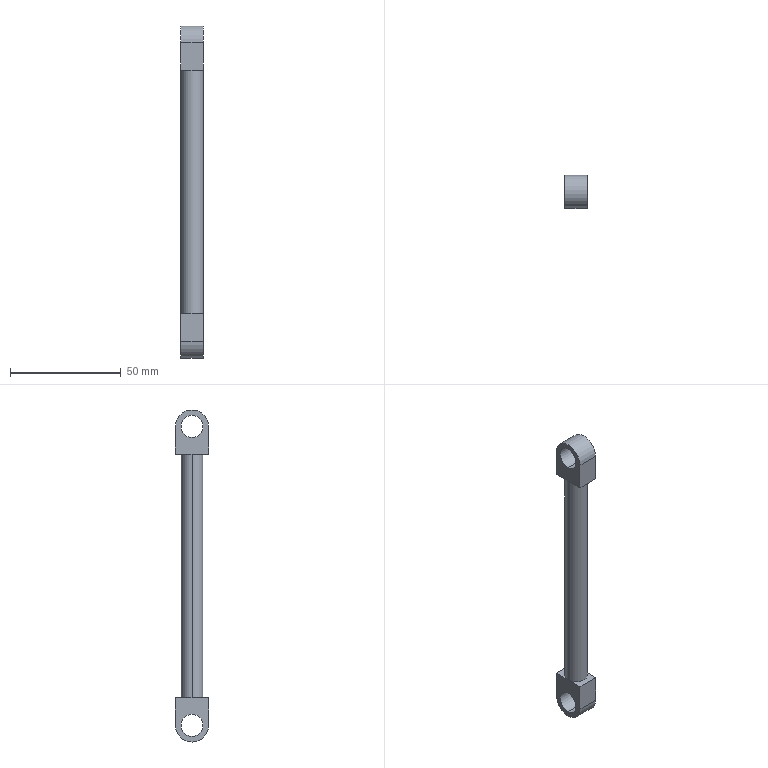Part | SolidWorks | features ICE 3, Extrusion 1 | 1 solid | 21 faces | box 10 x 15 x 150 mm | volume 12586 mm3 | plane 12 | cylinder 9 | commonest cylinder face diameters 10 x6 15 x3
STEP:
#1=CARTESIAN_POINT('',(-5.,0.,-7.5));
#2=VERTEX_POINT('',#1);
#3=CARTESIAN_POINT('',(-5.,0.,-17.5));
#4=VERTEX_POINT('',#3);
#5=CARTESIAN_POINT('',(-5.,0.,-12.5));
#6=DIRECTION('',(1.,0.,0.));
#7=DIRECTION('',(0.,0.,-1.));
#8=AXIS2_PLACEMENT_3D('',#5,#6,#7);
#9=CIRCLE('',#8,5.);
#10=EDGE_CURVE('',#2,#4,#9,.T.);
#11=ORIENTED_EDGE('',*,*,#10,.F.);
#12=CARTESIAN_POINT('',(5.,0.,-7.5));
#13=VERTEX_POINT('',#12);
#14=CARTESIAN_POINT('',(-5.,0.,-7.5));
#15=DIRECTION('',(1.,0.,0.));
#16=VECTOR('',#15,1000.);
#17=LINE('',#14,#16);
#18=EDGE_CURVE('',#2,#13,#17,.T.);
#19=ORIENTED_EDGE('',*,*,#18,.T.);
#20=CARTESIAN_POINT('',(5.,0.,-17.5));
#21=VERTEX_POINT('',#20);
#22=CARTESIAN_POINT('',(5.,0.,-12.5));
#23=DIRECTION('',(1.,0.,0.));
#24=DIRECTION('',(0.,0.,-1.));
#25=AXIS2_PLACEMENT_3D('',#22,#23,#24);
#26=CIRCLE('',#25,5.);
#27=EDGE_CURVE('',#13,#21,#26,.T.);
#28=ORIENTED_EDGE('',*,*,#27,.T.);
#29=CARTESIAN_POINT('',(-5.,0.,-17.5));
#30=DIRECTION('',(1.,0.,0.));
#31=VECTOR('',#30,1000.);
#32=LINE('',#29,#31);
#33=EDGE_CURVE('',#4,#21,#32,.T.);
#34=ORIENTED_EDGE('',*,*,#33,.F.);
#35=EDGE_LOOP('',(#11,#19,#28,#34));
#36=FACE_OUTER_BOUND('',#35,.T.);
#37=CARTESIAN_POINT('',(-5.,0.,-12.5));
#38=DIRECTION('',(1.,0.,0.));
#39=DIRECTION('',(0.,0.,-1.));
#40=AXIS2_PLACEMENT_3D('',#37,#38,#39);
#41=CYLINDRICAL_SURFACE('',#40,5.);
#42=ADVANCED_FACE('',(#36),#41,.F.);
#43=CARTESIAN_POINT('',(-5.,0.,-20.));
#44=VERTEX_POINT('',#43);
#45=CARTESIAN_POINT('',(-5.,-7.5,-12.5));
#46=VERTEX_POINT('',#45);
#47=CARTESIAN_POINT('',(-5.,0.,-12.5));
#48=DIRECTION('',(-1.,0.,0.));
#49=DIRECTION('',(0.,0.,-1.));
#50=AXIS2_PLACEMENT_3D('',#47,#48,#49);
#51=CIRCLE('',#50,7.5);
#52=EDGE_CURVE('',#44,#46,#51,.T.);
#53=ORIENTED_EDGE('',*,*,#52,.F.);
#54=CARTESIAN_POINT('',(5.,0.,-20.));
#55=VERTEX_POINT('',#54);
#56=CARTESIAN_POINT('',(-5.,0.,-20.));
#57=DIRECTION('',(1.,0.,0.));
#58=VECTOR('',#57,1000.);
#59=LINE('',#56,#58);
#60=EDGE_CURVE('',#44,#55,#59,.T.);
#61=ORIENTED_EDGE('',*,*,#60,.T.);
#62=CARTESIAN_POINT('',(5.,-7.5,-12.5));
#63=VERTEX_POINT('',#62);
#64=CARTESIAN_POINT('',(5.,0.,-12.5));
#65=DIRECTION('',(-1.,0.,0.));
#66=DIRECTION('',(0.,0.,-1.));
#67=AXIS2_PLACEMENT_3D('',#64,#65,#66);
#68=CIRCLE('',#67,7.5);
#69=EDGE_CURVE('',#55,#63,#68,.T.);
#70=ORIENTED_EDGE('',*,*,#69,.T.);
#71=CARTESIAN_POINT('',(-5.,-7.5,-12.5));
#72=DIRECTION('',(1.,0.,0.));
#73=VECTOR('',#72,1000.);
#74=LINE('',#71,#73);
#75=EDGE_CURVE('',#46,#63,#74,.T.);
#76=ORIENTED_EDGE('',*,*,#75,.F.);
#77=EDGE_LOOP('',(#53,#61,#70,#76));
#78=FACE_OUTER_BOUND('',#77,.T.);
#79=CARTESIAN_POINT('',(-5.,0.,-12.5));
#80=DIRECTION('',(1.,0.,0.));
#81=DIRECTION('',(0.,0.,-1.));
#82=AXIS2_PLACEMENT_3D('',#79,#80,#81);
#83=CYLINDRICAL_SURFACE('',#82,7.5);
#84=ADVANCED_FACE('',(#78),#83,.T.);
#85=CARTESIAN_POINT('',(-5.,0.,127.5));
#86=VERTEX_POINT('',#85);
#87=CARTESIAN_POINT('',(-5.,0.,117.5));
#88=VERTEX_POINT('',#87);
#89=CARTESIAN_POINT('',(-5.,0.,122.5));
#90=DIRECTION('',(1.,0.,0.));
#91=DIRECTION('',(0.,0.,-1.));
#92=AXIS2_PLACEMENT_3D('',#89,#90,#91);
#93=CIRCLE('',#92,5.);
#94=EDGE_CURVE('',#86,#88,#93,.T.);
#95=ORIENTED_EDGE('',*,*,#94,.F.);
#96=CARTESIAN_POINT('',(5.,0.,127.5));
#97=VERTEX_POINT('',#96);
#98=CARTESIAN_POINT('',(-5.,0.,127.5));
#99=DIRECTION('',(1.,0.,0.));
#100=VECTOR('',#99,1000.);
#101=LINE('',#98,#100);
#102=EDGE_CURVE('',#86,#97,#101,.T.);
#103=ORIENTED_EDGE('',*,*,#102,.T.);
#104=CARTESIAN_POINT('',(5.,0.,117.5));
#105=VERTEX_POINT('',#104);
#106=CARTESIAN_POINT('',(5.,0.,122.5));
#107=DIRECTION('',(1.,0.,0.));
#108=DIRECTION('',(0.,0.,-1.));
#109=AXIS2_PLACEMENT_3D('',#106,#107,#108);
#110=CIRCLE('',#109,5.);
#111=EDGE_CURVE('',#97,#105,#110,.T.);
#112=ORIENTED_EDGE('',*,*,#111,.T.);
#113=CARTESIAN_POINT('',(-5.,0.,117.5));
#114=DIRECTION('',(1.,0.,0.));
#115=VECTOR('',#114,1000.);
#116=LINE('',#113,#115);
#117=EDGE_CURVE('',#88,#105,#116,.T.);
#118=ORIENTED_EDGE('',*,*,#117,.F.);
#119=EDGE_LOOP('',(#95,#103,#112,#118));
#120=FACE_OUTER_BOUND('',#119,.T.);
#121=CARTESIAN_POINT('',(-5.,0.,122.5));
#122=DIRECTION('',(1.,0.,0.));
#123=DIRECTION('',(0.,0.,-1.));
#124=AXIS2_PLACEMENT_3D('',#121,#122,#123);
#125=CYLINDRICAL_SURFACE('',#124,5.);
#126=ADVANCED_FACE('',(#120),#125,.F.);
#127=CARTESIAN_POINT('',(5.,0.,110.));
#128=VERTEX_POINT('',#127);
#129=CARTESIAN_POINT('',(-5.,0.,110.));
#130=VERTEX_POINT('',#129);
#131=CARTESIAN_POINT('',(0.,0.,110.));
#132=DIRECTION('',(0.,0.,1.));
#133=DIRECTION('',(1.,0.,0.));
#134=AXIS2_PLACEMENT_3D('',#131,#132,#133);
#135=CIRCLE('',#134,5.);
#136=EDGE_CURVE('',#128,#130,#135,.T.);
#137=ORIENTED_EDGE('',*,*,#136,.F.);
#138=CARTESIAN_POINT('',(5.,0.,0.));
#139=VERTEX_POINT('',#138);
#140=CARTESIAN_POINT('',(5.,0.,110.));
#141=DIRECTION('',(0.,0.,-1.));
#142=VECTOR('',#141,1000.);
#143=LINE('',#140,#142);
#144=EDGE_CURVE('',#128,#139,#143,.T.);
#145=ORIENTED_EDGE('',*,*,#144,.T.);
#146=CARTESIAN_POINT('',(-5.,0.,0.));
#147=VERTEX_POINT('',#146);
#148=CARTESIAN_POINT('',(0.,0.,0.));
#149=DIRECTION('',(0.,0.,1.));
#150=DIRECTION('',(1.,0.,0.));
#151=AXIS2_PLACEMENT_3D('',#148,#149,#150);
#152=CIRCLE('',#151,5.);
#153=EDGE_CURVE('',#139,#147,#152,.T.);
#154=ORIENTED_EDGE('',*,*,#153,.T.);
#155=CARTESIAN_POINT('',(-5.,0.,110.));
#156=DIRECTION('',(0.,0.,-1.));
#157=VECTOR('',#156,1000.);
#158=LINE('',#155,#157);
#159=EDGE_CURVE('',#130,#147,#158,.T.);
#160=ORIENTED_EDGE('',*,*,#159,.F.);
#161=EDGE_LOOP('',(#137,#145,#154,#160));
#162=FACE_OUTER_BOUND('',#161,.T.);
#163=CARTESIAN_POINT('',(0.,0.,110.));
#164=DIRECTION('',(0.,0.,-1.));
#165=DIRECTION('',(-1.,0.,0.));
#166=AXIS2_PLACEMENT_3D('',#163,#164,#165);
#167=CYLINDRICAL_SURFACE('',#166,5.);
#168=ADVANCED_FACE('',(#162),#167,.T.);
#169=CARTESIAN_POINT('',(5.,-7.5,122.5));
#170=VERTEX_POINT('',#169);
#171=CARTESIAN_POINT('',(5.,7.5,122.5));
#172=VERTEX_POINT('',#171);
#173=CARTESIAN_POINT('',(5.,0.,122.5));
#174=DIRECTION('',(-1.,0.,0.));
#175=DIRECTION('',(0.,0.,-1.));
#176=AXIS2_PLACEMENT_3D('',#173,#174,#175);
#177=CIRCLE('',#176,7.5);
#178=EDGE_CURVE('',#170,#172,#177,.T.);
#179=ORIENTED_EDGE('',*,*,#178,.F.);
#180=CARTESIAN_POINT('',(5.,-7.5,110.));
#181=VERTEX_POINT('',#180);
#182=CARTESIAN_POINT('',(5.,-7.5,130.));
#183=DIRECTION('',(0.,0.,-1.));
#184=VECTOR('',#183,1000.);
#185=LINE('',#182,#184);
#186=EDGE_CURVE('',#170,#181,#185,.T.);
#187=ORIENTED_EDGE('',*,*,#186,.T.);
#188=CARTESIAN_POINT('',(5.,-7.5,110.));
#189=DIRECTION('',(0.,1.,0.));
#190=VECTOR('',#189,1000.);
#191=LINE('',#188,#190);
#192=EDGE_CURVE('',#181,#128,#191,.T.);
#193=ORIENTED_EDGE('',*,*,#192,.T.);
#194=CARTESIAN_POINT('',(5.,7.5,110.));
#195=VERTEX_POINT('',#194);
#196=CARTESIAN_POINT('',(5.,-7.5,110.));
#197=DIRECTION('',(0.,1.,0.));
#198=VECTOR('',#197,1000.);
#199=LINE('',#196,#198);
#200=EDGE_CURVE('',#128,#195,#199,.T.);
#201=ORIENTED_EDGE('',*,*,#200,.T.);
#202=CARTESIAN_POINT('',(5.,7.5,130.));
#203=DIRECTION('',(0.,0.,-1.));
#204=VECTOR('',#203,1000.);
#205=LINE('',#202,#204);
#206=EDGE_CURVE('',#172,#195,#205,.T.);
#207=ORIENTED_EDGE('',*,*,#206,.F.);
#208=EDGE_LOOP('',(#179,#187,#193,#201,#207));
#209=FACE_OUTER_BOUND('',#208,.T.);
#210=CARTESIAN_POINT('',(5.,0.,122.5));
#211=DIRECTION('',(1.,0.,0.));
#212=DIRECTION('',(0.,0.,-1.));
#213=AXIS2_PLACEMENT_3D('',#210,#211,#212);
#214=CIRCLE('',#213,5.);
#215=EDGE_CURVE('',#105,#97,#214,.T.);
#216=ORIENTED_EDGE('',*,*,#215,.F.);
#217=ORIENTED_EDGE('',*,*,#111,.F.);
#218=EDGE_LOOP('',(#216,#217));
#219=FACE_BOUND('',#218,.T.);
#220=CARTESIAN_POINT('',(5.,-7.5,130.));
#221=DIRECTION('',(-1.,0.,0.));
#222=DIRECTION('',(0.,0.,1.));
#223=AXIS2_PLACEMENT_3D('',#220,#221,#222);
#224=PLANE('',#223);
#225=ADVANCED_FACE('',(#209,#219),#224,.F.);
#226=CARTESIAN_POINT('',(-5.,-7.5,122.5));
#227=VERTEX_POINT('',#226);
#228=CARTESIAN_POINT('',(-5.,-7.5,110.));
#229=VERTEX_POINT('',#228);
#230=CARTESIAN_POINT('',(-5.,-7.5,130.));
#231=DIRECTION('',(0.,0.,-1.));
#232=VECTOR('',#231,1000.);
#233=LINE('',#230,#232);
#234=EDGE_CURVE('',#227,#229,#233,.T.);
#235=ORIENTED_EDGE('',*,*,#234,.F.);
#236=CARTESIAN_POINT('',(-5.,7.5,122.5));
#237=VERTEX_POINT('',#236);
#238=CARTESIAN_POINT('',(-5.,0.,122.5));
#239=DIRECTION('',(-1.,0.,0.));
#240=DIRECTION('',(0.,0.,-1.));
#241=AXIS2_PLACEMENT_3D('',#238,#239,#240);
#242=CIRCLE('',#241,7.5);
#243=EDGE_CURVE('',#227,#237,#242,.T.);
#244=ORIENTED_EDGE('',*,*,#243,.T.);
#245=CARTESIAN_POINT('',(-5.,7.5,110.));
#246=VERTEX_POINT('',#245);
#247=CARTESIAN_POINT('',(-5.,7.5,130.));
#248=DIRECTION('',(0.,0.,-1.));
#249=VECTOR('',#248,1000.);
#250=LINE('',#247,#249);
#251=EDGE_CURVE('',#237,#246,#250,.T.);
#252=ORIENTED_EDGE('',*,*,#251,.T.);
#253=CARTESIAN_POINT('',(-5.,-7.5,110.));
#254=DIRECTION('',(0.,-1.,0.));
#255=VECTOR('',#254,1000.);
#256=LINE('',#253,#255);
#257=EDGE_CURVE('',#246,#130,#256,.T.);
#258=ORIENTED_EDGE('',*,*,#257,.T.);
#259=CARTESIAN_POINT('',(-5.,-7.5,110.));
#260=DIRECTION('',(0.,-1.,0.));
#261=VECTOR('',#260,1000.);
#262=LINE('',#259,#261);
#263=EDGE_CURVE('',#130,#229,#262,.T.);
#264=ORIENTED_EDGE('',*,*,#263,.T.);
#265=EDGE_LOOP('',(#235,#244,#252,#258,#264));
#266=FACE_OUTER_BOUND('',#265,.T.);
#267=CARTESIAN_POINT('',(-5.,0.,122.5));
#268=DIRECTION('',(1.,0.,0.));
#269=DIRECTION('',(0.,0.,-1.));
#270=AXIS2_PLACEMENT_3D('',#267,#268,#269);
#271=CIRCLE('',#270,5.);
#272=EDGE_CURVE('',#88,#86,#271,.T.);
#273=ORIENTED_EDGE('',*,*,#272,.T.);
#274=ORIENTED_EDGE('',*,*,#94,.T.);
#275=EDGE_LOOP('',(#273,#274));
#276=FACE_BOUND('',#275,.T.);
#277=CARTESIAN_POINT('',(-5.,-7.5,130.));
#278=DIRECTION('',(1.,0.,0.));
#279=DIRECTION('',(0.,0.,-1.));
#280=AXIS2_PLACEMENT_3D('',#277,#278,#279);
#281=PLANE('',#280);
#282=ADVANCED_FACE('',(#266,#276),#281,.F.);
#283=ORIENTED_EDGE('',*,*,#144,.F.);
#284=CARTESIAN_POINT('',(0.,0.,110.));
#285=DIRECTION('',(0.,0.,1.));
#286=DIRECTION('',(1.,0.,0.));
#287=AXIS2_PLACEMENT_3D('',#284,#285,#286);
#288=CIRCLE('',#287,5.);
#289=EDGE_CURVE('',#130,#128,#288,.T.);
#290=ORIENTED_EDGE('',*,*,#289,.F.);
#291=ORIENTED_EDGE('',*,*,#159,.T.);
#292=CARTESIAN_POINT('',(0.,0.,0.));
#293=DIRECTION('',(0.,0.,1.));
#294=DIRECTION('',(1.,0.,0.));
#295=AXIS2_PLACEMENT_3D('',#292,#293,#294);
#296=CIRCLE('',#295,5.);
#297=EDGE_CURVE('',#147,#139,#296,.T.);
#298=ORIENTED_EDGE('',*,*,#297,.T.);
#299=EDGE_LOOP('',(#283,#290,#291,#298));
#300=FACE_OUTER_BOUND('',#299,.T.);
#301=CARTESIAN_POINT('',(0.,0.,110.));
#302=DIRECTION('',(0.,0.,-1.));
#303=DIRECTION('',(-1.,0.,0.));
#304=AXIS2_PLACEMENT_3D('',#301,#302,#303);
#305=CYLINDRICAL_SURFACE('',#304,5.);
#306=ADVANCED_FACE('',(#300),#305,.T.);
#307=ORIENTED_EDGE('',*,*,#153,.F.);
#308=CARTESIAN_POINT('',(5.,7.5,0.));
#309=VERTEX_POINT('',#308);
#310=CARTESIAN_POINT('',(5.,7.5,0.));
#311=DIRECTION('',(0.,-1.,0.));
#312=VECTOR('',#311,1000.);
#313=LINE('',#310,#312);
#314=EDGE_CURVE('',#309,#139,#313,.T.);
#315=ORIENTED_EDGE('',*,*,#314,.F.);
#316=CARTESIAN_POINT('',(-5.,7.5,0.));
#317=VERTEX_POINT('',#316);
#318=CARTESIAN_POINT('',(5.,7.5,0.));
#319=DIRECTION('',(1.,0.,0.));
#320=VECTOR('',#319,1000.);
#321=LINE('',#318,#320);
#322=EDGE_CURVE('',#317,#309,#321,.T.);
#323=ORIENTED_EDGE('',*,*,#322,.F.);
#324=CARTESIAN_POINT('',(-5.,7.5,0.));
#325=DIRECTION('',(0.,1.,0.));
#326=VECTOR('',#325,1000.);
#327=LINE('',#324,#326);
#328=EDGE_CURVE('',#147,#317,#327,.T.);
#329=ORIENTED_EDGE('',*,*,#328,.F.);
#330=EDGE_LOOP('',(#307,#315,#323,#329));
#331=FACE_OUTER_BOUND('',#330,.T.);
#332=CARTESIAN_POINT('',(0.,0.,0.));
#333=DIRECTION('',(0.,0.,-1.));
#334=DIRECTION('',(-1.,0.,0.));
#335=AXIS2_PLACEMENT_3D('',#332,#333,#334);
#336=PLANE('',#335);
#337=ADVANCED_FACE('',(#331),#336,.F.);
#338=CARTESIAN_POINT('',(-5.,0.,-12.5));
#339=DIRECTION('',(1.,0.,0.));
#340=DIRECTION('',(0.,0.,-1.));
#341=AXIS2_PLACEMENT_3D('',#338,#339,#340);
#342=CIRCLE('',#341,5.);
#343=EDGE_CURVE('',#4,#2,#342,.T.);
#344=ORIENTED_EDGE('',*,*,#343,.T.);
#345=ORIENTED_EDGE('',*,*,#10,.T.);
#346=EDGE_LOOP('',(#344,#345));
#347=FACE_BOUND('',#346,.T.);
#348=CARTESIAN_POINT('',(-5.,7.5,-12.5));
#349=VERTEX_POINT('',#348);
#350=CARTESIAN_POINT('',(-5.,7.5,-20.));
#351=DIRECTION('',(0.,0.,1.));
#352=VECTOR('',#351,1000.);
#353=LINE('',#350,#352);
#354=EDGE_CURVE('',#349,#317,#353,.T.);
#355=ORIENTED_EDGE('',*,*,#354,.F.);
#356=CARTESIAN_POINT('',(-5.,0.,-12.5));
#357=DIRECTION('',(-1.,0.,0.));
#358=DIRECTION('',(0.,0.,-1.));
#359=AXIS2_PLACEMENT_3D('',#356,#357,#358);
#360=CIRCLE('',#359,7.5);
#361=EDGE_CURVE('',#349,#44,#360,.T.);
#362=ORIENTED_EDGE('',*,*,#361,.T.);
#363=ORIENTED_EDGE('',*,*,#52,.T.);
#364=CARTESIAN_POINT('',(-5.,-7.5,0.));
#365=VERTEX_POINT('',#364);
#366=CARTESIAN_POINT('',(-5.,-7.5,-20.));
#367=DIRECTION('',(0.,0.,1.));
#368=VECTOR('',#367,1000.);
#369=LINE('',#366,#368);
#370=EDGE_CURVE('',#46,#365,#369,.T.);
#371=ORIENTED_EDGE('',*,*,#370,.T.);
#372=CARTESIAN_POINT('',(-5.,7.5,0.));
#373=DIRECTION('',(0.,1.,0.));
#374=VECTOR('',#373,1000.);
#375=LINE('',#372,#374);
#376=EDGE_CURVE('',#365,#147,#375,.T.);
#377=ORIENTED_EDGE('',*,*,#376,.T.);
#378=ORIENTED_EDGE('',*,*,#328,.T.);
#379=EDGE_LOOP('',(#355,#362,#363,#371,#377,#378));
#380=FACE_OUTER_BOUND('',#379,.T.);
#381=CARTESIAN_POINT('',(-5.,7.5,-20.));
#382=DIRECTION('',(1.,0.,0.));
#383=DIRECTION('',(0.,1.,0.));
#384=AXIS2_PLACEMENT_3D('',#381,#382,#383);
#385=PLANE('',#384);
#386=ADVANCED_FACE('',(#347,#380),#385,.F.);
#387=CARTESIAN_POINT('',(5.,7.5,-12.5));
#388=VERTEX_POINT('',#387);
#389=CARTESIAN_POINT('',(5.,7.5,-20.));
#390=DIRECTION('',(0.,0.,1.));
#391=VECTOR('',#390,1000.);
#392=LINE('',#389,#391);
#393=EDGE_CURVE('',#388,#309,#392,.T.);
#394=ORIENTED_EDGE('',*,*,#393,.F.);
#395=CARTESIAN_POINT('',(-5.,7.5,-12.5));
#396=DIRECTION('',(1.,0.,0.));
#397=VECTOR('',#396,1000.);
#398=LINE('',#395,#397);
#399=EDGE_CURVE('',#349,#388,#398,.T.);
#400=ORIENTED_EDGE('',*,*,#399,.F.);
#401=ORIENTED_EDGE('',*,*,#354,.T.);
#402=ORIENTED_EDGE('',*,*,#322,.T.);
#403=EDGE_LOOP('',(#394,#400,#401,#402));
#404=FACE_OUTER_BOUND('',#403,.T.);
#405=CARTESIAN_POINT('',(5.,7.5,-20.));
#406=DIRECTION('',(0.,-1.,0.));
#407=DIRECTION('',(0.,0.,-1.));
#408=AXIS2_PLACEMENT_3D('',#405,#406,#407);
#409=PLANE('',#408);
#410=ADVANCED_FACE('',(#404),#409,.F.);
#411=CARTESIAN_POINT('',(5.,0.,-12.5));
#412=DIRECTION('',(1.,0.,0.));
#413=DIRECTION('',(0.,0.,-1.));
#414=AXIS2_PLACEMENT_3D('',#411,#412,#413);
#415=CIRCLE('',#414,5.);
#416=EDGE_CURVE('',#21,#13,#415,.T.);
#417=ORIENTED_EDGE('',*,*,#416,.F.);
#418=ORIENTED_EDGE('',*,*,#27,.F.);
#419=EDGE_LOOP('',(#417,#418));
#420=FACE_BOUND('',#419,.T.);
#421=CARTESIAN_POINT('',(5.,-7.5,0.));
#422=VERTEX_POINT('',#421);
#423=CARTESIAN_POINT('',(5.,-7.5,-20.));
#424=DIRECTION('',(0.,0.,1.));
#425=VECTOR('',#424,1000.);
#426=LINE('',#423,#425);
#427=EDGE_CURVE('',#63,#422,#426,.T.);
#428=ORIENTED_EDGE('',*,*,#427,.F.);
#429=ORIENTED_EDGE('',*,*,#69,.F.);
#430=CARTESIAN_POINT('',(5.,0.,-12.5));
#431=DIRECTION('',(-1.,0.,0.));
#432=DIRECTION('',(0.,0.,-1.));
#433=AXIS2_PLACEMENT_3D('',#430,#431,#432);
#434=CIRCLE('',#433,7.5);
#435=EDGE_CURVE('',#388,#55,#434,.T.);
#436=ORIENTED_EDGE('',*,*,#435,.F.);
#437=ORIENTED_EDGE('',*,*,#393,.T.);
#438=ORIENTED_EDGE('',*,*,#314,.T.);
#439=CARTESIAN_POINT('',(5.,7.5,0.));
#440=DIRECTION('',(0.,-1.,0.));
#441=VECTOR('',#440,1000.);
#442=LINE('',#439,#441);
#443=EDGE_CURVE('',#139,#422,#442,.T.);
#444=ORIENTED_EDGE('',*,*,#443,.T.);
#445=EDGE_LOOP('',(#428,#429,#436,#437,#438,#444));
#446=FACE_OUTER_BOUND('',#445,.T.);
#447=CARTESIAN_POINT('',(5.,7.5,-20.));
#448=DIRECTION('',(-1.,0.,0.));
#449=DIRECTION('',(0.,-1.,0.));
#450=AXIS2_PLACEMENT_3D('',#447,#448,#449);
#451=PLANE('',#450);
#452=ADVANCED_FACE('',(#420,#446),#451,.F.);
#453=ORIENTED_EDGE('',*,*,#370,.F.);
#454=ORIENTED_EDGE('',*,*,#75,.T.);
#455=ORIENTED_EDGE('',*,*,#427,.T.);
#456=CARTESIAN_POINT('',(5.,-7.5,0.));
#457=DIRECTION('',(-1.,0.,0.));
#458=VECTOR('',#457,1000.);
#459=LINE('',#456,#458);
#460=EDGE_CURVE('',#422,#365,#459,.T.);
#461=ORIENTED_EDGE('',*,*,#460,.T.);
#462=EDGE_LOOP('',(#453,#454,#455,#461));
#463=FACE_OUTER_BOUND('',#462,.T.);
#464=CARTESIAN_POINT('',(5.,-7.5,-20.));
#465=DIRECTION('',(0.,1.,0.));
#466=DIRECTION('',(0.,0.,1.));
#467=AXIS2_PLACEMENT_3D('',#464,#465,#466);
#468=PLANE('',#467);
#469=ADVANCED_FACE('',(#463),#468,.F.);
#470=ORIENTED_EDGE('',*,*,#297,.F.);
#471=ORIENTED_EDGE('',*,*,#376,.F.);
#472=ORIENTED_EDGE('',*,*,#460,.F.);
#473=ORIENTED_EDGE('',*,*,#443,.F.);
#474=EDGE_LOOP('',(#470,#471,#472,#473));
#475=FACE_OUTER_BOUND('',#474,.T.);
#476=CARTESIAN_POINT('',(0.,0.,0.));
#477=DIRECTION('',(0.,0.,-1.));
#478=DIRECTION('',(-1.,0.,0.));
#479=AXIS2_PLACEMENT_3D('',#476,#477,#478);
#480=PLANE('',#479);
#481=ADVANCED_FACE('',(#475),#480,.F.);
#482=ORIENTED_EDGE('',*,*,#200,.F.);
#483=ORIENTED_EDGE('',*,*,#136,.T.);
#484=ORIENTED_EDGE('',*,*,#257,.F.);
#485=CARTESIAN_POINT('',(-5.,7.5,110.));
#486=DIRECTION('',(-1.,0.,0.));
#487=VECTOR('',#486,1000.);
#488=LINE('',#485,#487);
#489=EDGE_CURVE('',#195,#246,#488,.T.);
#490=ORIENTED_EDGE('',*,*,#489,.F.);
#491=EDGE_LOOP('',(#482,#483,#484,#490));
#492=FACE_OUTER_BOUND('',#491,.T.);
#493=CARTESIAN_POINT('',(0.,0.,110.));
#494=DIRECTION('',(0.,0.,-1.));
#495=DIRECTION('',(-1.,0.,0.));
#496=AXIS2_PLACEMENT_3D('',#493,#494,#495);
#497=PLANE('',#496);
#498=ADVANCED_FACE('',(#492),#497,.T.);
#499=ORIENTED_EDGE('',*,*,#251,.F.);
#500=CARTESIAN_POINT('',(-5.,7.5,122.5));
#501=DIRECTION('',(1.,0.,0.));
#502=VECTOR('',#501,1000.);
#503=LINE('',#500,#502);
#504=EDGE_CURVE('',#237,#172,#503,.T.);
#505=ORIENTED_EDGE('',*,*,#504,.T.);
#506=ORIENTED_EDGE('',*,*,#206,.T.);
#507=ORIENTED_EDGE('',*,*,#489,.T.);
#508=EDGE_LOOP('',(#499,#505,#506,#507));
#509=FACE_OUTER_BOUND('',#508,.T.);
#510=CARTESIAN_POINT('',(-5.,7.5,130.));
#511=DIRECTION('',(0.,-1.,0.));
#512=DIRECTION('',(0.,0.,-1.));
#513=AXIS2_PLACEMENT_3D('',#510,#511,#512);
#514=PLANE('',#513);
#515=ADVANCED_FACE('',(#509),#514,.F.);
#516=ORIENTED_EDGE('',*,*,#186,.F.);
#517=CARTESIAN_POINT('',(-5.,-7.5,122.5));
#518=DIRECTION('',(1.,0.,0.));
#519=VECTOR('',#518,1000.);
#520=LINE('',#517,#519);
#521=EDGE_CURVE('',#227,#170,#520,.T.);
#522=ORIENTED_EDGE('',*,*,#521,.F.);
#523=ORIENTED_EDGE('',*,*,#234,.T.);
#524=CARTESIAN_POINT('',(-5.,-7.5,110.));
#525=DIRECTION('',(1.,0.,0.));
#526=VECTOR('',#525,1000.);
#527=LINE('',#524,#526);
#528=EDGE_CURVE('',#229,#181,#527,.T.);
#529=ORIENTED_EDGE('',*,*,#528,.T.);
#530=EDGE_LOOP('',(#516,#522,#523,#529));
#531=FACE_OUTER_BOUND('',#530,.T.);
#532=CARTESIAN_POINT('',(-5.,-7.5,130.));
#533=DIRECTION('',(0.,1.,0.));
#534=DIRECTION('',(0.,0.,1.));
#535=AXIS2_PLACEMENT_3D('',#532,#533,#534);
#536=PLANE('',#535);
#537=ADVANCED_FACE('',(#531),#536,.F.);
#538=ORIENTED_EDGE('',*,*,#263,.F.);
#539=ORIENTED_EDGE('',*,*,#289,.T.);
#540=ORIENTED_EDGE('',*,*,#192,.F.);
#541=ORIENTED_EDGE('',*,*,#528,.F.);
#542=EDGE_LOOP('',(#538,#539,#540,#541));
#543=FACE_OUTER_BOUND('',#542,.T.);
#544=CARTESIAN_POINT('',(0.,0.,110.));
#545=DIRECTION('',(0.,0.,-1.));
#546=DIRECTION('',(-1.,0.,0.));
#547=AXIS2_PLACEMENT_3D('',#544,#545,#546);
#548=PLANE('',#547);
#549=ADVANCED_FACE('',(#543),#548,.T.);
#550=ORIENTED_EDGE('',*,*,#178,.T.);
#551=ORIENTED_EDGE('',*,*,#504,.F.);
#552=ORIENTED_EDGE('',*,*,#243,.F.);
#553=ORIENTED_EDGE('',*,*,#521,.T.);
#554=EDGE_LOOP('',(#550,#551,#552,#553));
#555=FACE_OUTER_BOUND('',#554,.T.);
#556=CARTESIAN_POINT('',(-5.,0.,122.5));
#557=DIRECTION('',(1.,0.,0.));
#558=DIRECTION('',(0.,0.,-1.));
#559=AXIS2_PLACEMENT_3D('',#556,#557,#558);
#560=CYLINDRICAL_SURFACE('',#559,7.5);
#561=ADVANCED_FACE('',(#555),#560,.T.);
#562=ORIENTED_EDGE('',*,*,#102,.F.);
#563=ORIENTED_EDGE('',*,*,#272,.F.);
#564=ORIENTED_EDGE('',*,*,#117,.T.);
#565=ORIENTED_EDGE('',*,*,#215,.T.);
#566=EDGE_LOOP('',(#562,#563,#564,#565));
#567=FACE_OUTER_BOUND('',#566,.T.);
#568=CARTESIAN_POINT('',(-5.,0.,122.5));
#569=DIRECTION('',(1.,0.,0.));
#570=DIRECTION('',(0.,0.,-1.));
#571=AXIS2_PLACEMENT_3D('',#568,#569,#570);
#572=CYLINDRICAL_SURFACE('',#571,5.);
#573=ADVANCED_FACE('',(#567),#572,.F.);
#574=ORIENTED_EDGE('',*,*,#60,.F.);
#575=ORIENTED_EDGE('',*,*,#361,.F.);
#576=ORIENTED_EDGE('',*,*,#399,.T.);
#577=ORIENTED_EDGE('',*,*,#435,.T.);
#578=EDGE_LOOP('',(#574,#575,#576,#577));
#579=FACE_OUTER_BOUND('',#578,.T.);
#580=CARTESIAN_POINT('',(-5.,0.,-12.5));
#581=DIRECTION('',(1.,0.,0.));
#582=DIRECTION('',(0.,0.,-1.));
#583=AXIS2_PLACEMENT_3D('',#580,#581,#582);
#584=CYLINDRICAL_SURFACE('',#583,7.5);
#585=ADVANCED_FACE('',(#579),#584,.T.);
#586=ORIENTED_EDGE('',*,*,#18,.F.);
#587=ORIENTED_EDGE('',*,*,#343,.F.);
#588=ORIENTED_EDGE('',*,*,#33,.T.);
#589=ORIENTED_EDGE('',*,*,#416,.T.);
#590=EDGE_LOOP('',(#586,#587,#588,#589));
#591=FACE_OUTER_BOUND('',#590,.T.);
#592=CARTESIAN_POINT('',(-5.,0.,-12.5));
#593=DIRECTION('',(1.,0.,0.));
#594=DIRECTION('',(0.,0.,-1.));
#595=AXIS2_PLACEMENT_3D('',#592,#593,#594);
#596=CYLINDRICAL_SURFACE('',#595,5.);
#597=ADVANCED_FACE('',(#591),#596,.F.);
#598=CLOSED_SHELL('',(#42,#84,#126,#168,#225,#282,#306,#337,#386,#410,#452,#469,#481,#498,#515,#537,#549,#561,#573,#585,#597));
#599=MANIFOLD_SOLID_BREP('',#598);
#600=CARTESIAN_POINT('',(0.,0.,0.));
#601=DIRECTION('',(0.,0.,1.));
#602=DIRECTION('',(1.,0.,0.));
#603=AXIS2_PLACEMENT_3D('',#600,#601,#602);
#604=(LENGTH_UNIT()NAMED_UNIT(*)SI_UNIT(.MILLI.,.METRE.));
#605=UNCERTAINTY_MEASURE_WITH_UNIT(LENGTH_MEASURE(0.00001),#604,'','');
#606=(NAMED_UNIT(*)PLANE_ANGLE_UNIT()SI_UNIT($,.RADIAN.));
#607=(NAMED_UNIT(*)SI_UNIT($,.STERADIAN.)SOLID_ANGLE_UNIT());
#608=(GEOMETRIC_REPRESENTATION_CONTEXT(3)GLOBAL_UNCERTAINTY_ASSIGNED_CONTEXT((#605))GLOBAL_UNIT_ASSIGNED_CONTEXT((#604,#606,#607))REPRESENTATION_CONTEXT('',''));
#609=ADVANCED_BREP_SHAPE_REPRESENTATION('',(#599,#603),#608);